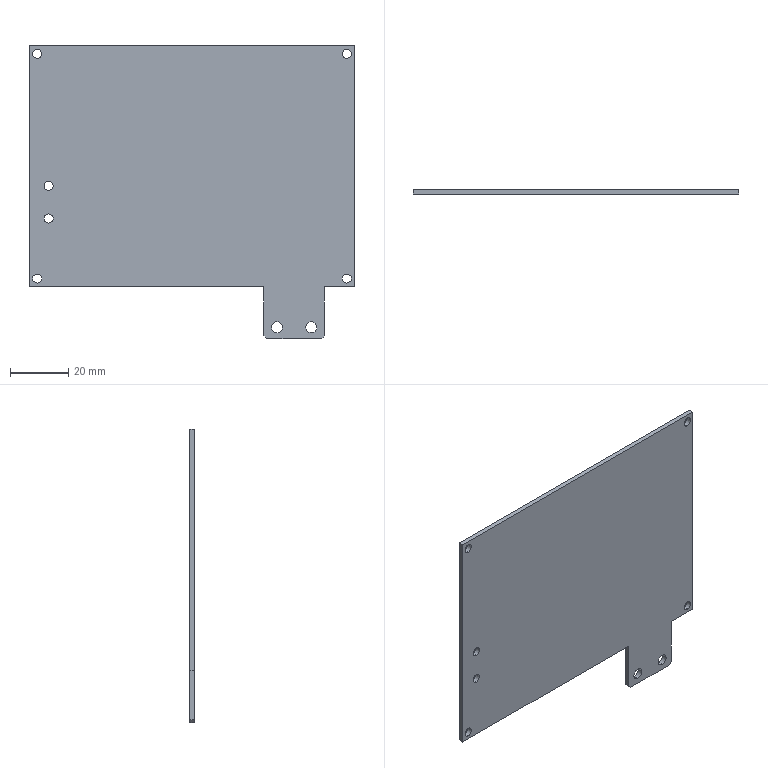Part | SolidWorks | features Extrusion 1 | 1 solid | 28 faces | box 111.5 x 1.7 x 100.35 mm | volume 16166 mm3 | cylinder 16 | plane 12 | commonest cylinder face diameters 3.1 x12 3.8 x4
STEP:
#1=CARTESIAN_POINT('',(-49.1,1.7,-8.3));
#2=VERTEX_POINT('',#1);
#3=CARTESIAN_POINT('',(-49.1,1.7,-5.2));
#4=VERTEX_POINT('',#3);
#5=CARTESIAN_POINT('',(-49.1,1.7,-6.75));
#6=DIRECTION('',(0.,1.,0.));
#7=DIRECTION('',(0.,0.,1.));
#8=AXIS2_PLACEMENT_3D('',#5,#6,#7);
#9=CIRCLE('',#8,1.55);
#10=EDGE_CURVE('',#2,#4,#9,.T.);
#11=ORIENTED_EDGE('',*,*,#10,.T.);
#12=CARTESIAN_POINT('',(-49.1,0.,-5.2));
#13=VERTEX_POINT('',#12);
#14=CARTESIAN_POINT('',(-49.1,1.7,-5.2));
#15=DIRECTION('',(0.,-1.,0.));
#16=VECTOR('',#15,1000.);
#17=LINE('',#14,#16);
#18=EDGE_CURVE('',#4,#13,#17,.T.);
#19=ORIENTED_EDGE('',*,*,#18,.T.);
#20=CARTESIAN_POINT('',(-49.1,0.,-8.3));
#21=VERTEX_POINT('',#20);
#22=CARTESIAN_POINT('',(-49.1,0.,-6.75));
#23=DIRECTION('',(0.,1.,0.));
#24=DIRECTION('',(0.,0.,1.));
#25=AXIS2_PLACEMENT_3D('',#22,#23,#24);
#26=CIRCLE('',#25,1.55);
#27=EDGE_CURVE('',#21,#13,#26,.T.);
#28=ORIENTED_EDGE('',*,*,#27,.F.);
#29=CARTESIAN_POINT('',(-49.1,1.7,-8.3));
#30=DIRECTION('',(0.,-1.,0.));
#31=VECTOR('',#30,1000.);
#32=LINE('',#29,#31);
#33=EDGE_CURVE('',#2,#21,#32,.T.);
#34=ORIENTED_EDGE('',*,*,#33,.F.);
#35=EDGE_LOOP('',(#11,#19,#28,#34));
#36=FACE_OUTER_BOUND('',#35,.T.);
#37=CARTESIAN_POINT('',(-49.1,1.7,-6.75));
#38=DIRECTION('',(0.,-1.,0.));
#39=DIRECTION('',(0.,0.,-1.));
#40=AXIS2_PLACEMENT_3D('',#37,#38,#39);
#41=CYLINDRICAL_SURFACE('',#40,1.55);
#42=ADVANCED_FACE('',(#36),#41,.F.);
#43=CARTESIAN_POINT('',(-49.1,1.7,-19.5));
#44=VERTEX_POINT('',#43);
#45=CARTESIAN_POINT('',(-49.1,1.7,-16.4));
#46=VERTEX_POINT('',#45);
#47=CARTESIAN_POINT('',(-49.1,1.7,-17.95));
#48=DIRECTION('',(0.,1.,0.));
#49=DIRECTION('',(0.,0.,1.));
#50=AXIS2_PLACEMENT_3D('',#47,#48,#49);
#51=CIRCLE('',#50,1.55);
#52=EDGE_CURVE('',#44,#46,#51,.T.);
#53=ORIENTED_EDGE('',*,*,#52,.T.);
#54=CARTESIAN_POINT('',(-49.1,0.,-16.4));
#55=VERTEX_POINT('',#54);
#56=CARTESIAN_POINT('',(-49.1,1.7,-16.4));
#57=DIRECTION('',(0.,-1.,0.));
#58=VECTOR('',#57,1000.);
#59=LINE('',#56,#58);
#60=EDGE_CURVE('',#46,#55,#59,.T.);
#61=ORIENTED_EDGE('',*,*,#60,.T.);
#62=CARTESIAN_POINT('',(-49.1,0.,-19.5));
#63=VERTEX_POINT('',#62);
#64=CARTESIAN_POINT('',(-49.1,0.,-17.95));
#65=DIRECTION('',(0.,1.,0.));
#66=DIRECTION('',(0.,0.,1.));
#67=AXIS2_PLACEMENT_3D('',#64,#65,#66);
#68=CIRCLE('',#67,1.55);
#69=EDGE_CURVE('',#63,#55,#68,.T.);
#70=ORIENTED_EDGE('',*,*,#69,.F.);
#71=CARTESIAN_POINT('',(-49.1,1.7,-19.5));
#72=DIRECTION('',(0.,-1.,0.));
#73=VECTOR('',#72,1000.);
#74=LINE('',#71,#73);
#75=EDGE_CURVE('',#44,#63,#74,.T.);
#76=ORIENTED_EDGE('',*,*,#75,.F.);
#77=EDGE_LOOP('',(#53,#61,#70,#76));
#78=FACE_OUTER_BOUND('',#77,.T.);
#79=CARTESIAN_POINT('',(-49.1,1.7,-17.95));
#80=DIRECTION('',(0.,-1.,0.));
#81=DIRECTION('',(0.,0.,-1.));
#82=AXIS2_PLACEMENT_3D('',#79,#80,#81);
#83=CYLINDRICAL_SURFACE('',#82,1.55);
#84=ADVANCED_FACE('',(#78),#83,.F.);
#85=CARTESIAN_POINT('',(40.875,1.7,-57.05));
#86=VERTEX_POINT('',#85);
#87=CARTESIAN_POINT('',(40.875,1.7,-53.25));
#88=VERTEX_POINT('',#87);
#89=CARTESIAN_POINT('',(40.875,1.7,-55.15));
#90=DIRECTION('',(0.,1.,0.));
#91=DIRECTION('',(0.,0.,-1.));
#92=AXIS2_PLACEMENT_3D('',#89,#90,#91);
#93=CIRCLE('',#92,1.9);
#94=EDGE_CURVE('',#86,#88,#93,.T.);
#95=ORIENTED_EDGE('',*,*,#94,.T.);
#96=CARTESIAN_POINT('',(40.875,0.,-53.25));
#97=VERTEX_POINT('',#96);
#98=CARTESIAN_POINT('',(40.875,1.7,-53.25));
#99=DIRECTION('',(0.,-1.,0.));
#100=VECTOR('',#99,1000.);
#101=LINE('',#98,#100);
#102=EDGE_CURVE('',#88,#97,#101,.T.);
#103=ORIENTED_EDGE('',*,*,#102,.T.);
#104=CARTESIAN_POINT('',(40.875,0.,-57.05));
#105=VERTEX_POINT('',#104);
#106=CARTESIAN_POINT('',(40.875,0.,-55.15));
#107=DIRECTION('',(0.,1.,0.));
#108=DIRECTION('',(0.,0.,-1.));
#109=AXIS2_PLACEMENT_3D('',#106,#107,#108);
#110=CIRCLE('',#109,1.9);
#111=EDGE_CURVE('',#105,#97,#110,.T.);
#112=ORIENTED_EDGE('',*,*,#111,.F.);
#113=CARTESIAN_POINT('',(40.875,1.7,-57.05));
#114=DIRECTION('',(0.,-1.,0.));
#115=VECTOR('',#114,1000.);
#116=LINE('',#113,#115);
#117=EDGE_CURVE('',#86,#105,#116,.T.);
#118=ORIENTED_EDGE('',*,*,#117,.F.);
#119=EDGE_LOOP('',(#95,#103,#112,#118));
#120=FACE_OUTER_BOUND('',#119,.T.);
#121=CARTESIAN_POINT('',(40.875,1.7,-55.15));
#122=DIRECTION('',(0.,-1.,0.));
#123=DIRECTION('',(0.,0.,-1.));
#124=AXIS2_PLACEMENT_3D('',#121,#122,#123);
#125=CYLINDRICAL_SURFACE('',#124,1.9);
#126=ADVANCED_FACE('',(#120),#125,.F.);
#127=CARTESIAN_POINT('',(29.075,1.7,-57.05));
#128=VERTEX_POINT('',#127);
#129=CARTESIAN_POINT('',(29.075,1.7,-53.25));
#130=VERTEX_POINT('',#129);
#131=CARTESIAN_POINT('',(29.075,1.7,-55.15));
#132=DIRECTION('',(0.,1.,0.));
#133=DIRECTION('',(0.,0.,1.));
#134=AXIS2_PLACEMENT_3D('',#131,#132,#133);
#135=CIRCLE('',#134,1.9);
#136=EDGE_CURVE('',#128,#130,#135,.T.);
#137=ORIENTED_EDGE('',*,*,#136,.T.);
#138=CARTESIAN_POINT('',(29.075,0.,-53.25));
#139=VERTEX_POINT('',#138);
#140=CARTESIAN_POINT('',(29.075,1.7,-53.25));
#141=DIRECTION('',(0.,-1.,0.));
#142=VECTOR('',#141,1000.);
#143=LINE('',#140,#142);
#144=EDGE_CURVE('',#130,#139,#143,.T.);
#145=ORIENTED_EDGE('',*,*,#144,.T.);
#146=CARTESIAN_POINT('',(29.075,0.,-57.05));
#147=VERTEX_POINT('',#146);
#148=CARTESIAN_POINT('',(29.075,0.,-55.15));
#149=DIRECTION('',(0.,1.,0.));
#150=DIRECTION('',(0.,0.,1.));
#151=AXIS2_PLACEMENT_3D('',#148,#149,#150);
#152=CIRCLE('',#151,1.9);
#153=EDGE_CURVE('',#147,#139,#152,.T.);
#154=ORIENTED_EDGE('',*,*,#153,.F.);
#155=CARTESIAN_POINT('',(29.075,1.7,-57.05));
#156=DIRECTION('',(0.,-1.,0.));
#157=VECTOR('',#156,1000.);
#158=LINE('',#155,#157);
#159=EDGE_CURVE('',#128,#147,#158,.T.);
#160=ORIENTED_EDGE('',*,*,#159,.F.);
#161=EDGE_LOOP('',(#137,#145,#154,#160));
#162=FACE_OUTER_BOUND('',#161,.T.);
#163=CARTESIAN_POINT('',(29.075,1.7,-55.15));
#164=DIRECTION('',(0.,-1.,0.));
#165=DIRECTION('',(0.,0.,-1.));
#166=AXIS2_PLACEMENT_3D('',#163,#164,#165);
#167=CYLINDRICAL_SURFACE('',#166,1.9);
#168=ADVANCED_FACE('',(#162),#167,.F.);
#169=CARTESIAN_POINT('',(-53.,1.7,36.95));
#170=VERTEX_POINT('',#169);
#171=CARTESIAN_POINT('',(-53.,1.7,40.05));
#172=VERTEX_POINT('',#171);
#173=CARTESIAN_POINT('',(-53.,1.7,38.5));
#174=DIRECTION('',(0.,1.,0.));
#175=DIRECTION('',(0.,0.,-1.));
#176=AXIS2_PLACEMENT_3D('',#173,#174,#175);
#177=CIRCLE('',#176,1.55);
#178=EDGE_CURVE('',#170,#172,#177,.T.);
#179=ORIENTED_EDGE('',*,*,#178,.T.);
#180=CARTESIAN_POINT('',(-53.,0.,40.05));
#181=VERTEX_POINT('',#180);
#182=CARTESIAN_POINT('',(-53.,1.7,40.05));
#183=DIRECTION('',(0.,-1.,0.));
#184=VECTOR('',#183,1000.);
#185=LINE('',#182,#184);
#186=EDGE_CURVE('',#172,#181,#185,.T.);
#187=ORIENTED_EDGE('',*,*,#186,.T.);
#188=CARTESIAN_POINT('',(-53.,0.,36.95));
#189=VERTEX_POINT('',#188);
#190=CARTESIAN_POINT('',(-53.,0.,38.5));
#191=DIRECTION('',(0.,1.,0.));
#192=DIRECTION('',(0.,0.,-1.));
#193=AXIS2_PLACEMENT_3D('',#190,#191,#192);
#194=CIRCLE('',#193,1.55);
#195=EDGE_CURVE('',#189,#181,#194,.T.);
#196=ORIENTED_EDGE('',*,*,#195,.F.);
#197=CARTESIAN_POINT('',(-53.,1.7,36.95));
#198=DIRECTION('',(0.,-1.,0.));
#199=VECTOR('',#198,1000.);
#200=LINE('',#197,#199);
#201=EDGE_CURVE('',#170,#189,#200,.T.);
#202=ORIENTED_EDGE('',*,*,#201,.F.);
#203=EDGE_LOOP('',(#179,#187,#196,#202));
#204=FACE_OUTER_BOUND('',#203,.T.);
#205=CARTESIAN_POINT('',(-53.,1.7,38.5));
#206=DIRECTION('',(0.,-1.,0.));
#207=DIRECTION('',(0.,0.,-1.));
#208=AXIS2_PLACEMENT_3D('',#205,#206,#207);
#209=CYLINDRICAL_SURFACE('',#208,1.55);
#210=ADVANCED_FACE('',(#204),#209,.F.);
#211=CARTESIAN_POINT('',(53.,1.7,36.95));
#212=VERTEX_POINT('',#211);
#213=CARTESIAN_POINT('',(53.,1.7,40.05));
#214=VERTEX_POINT('',#213);
#215=CARTESIAN_POINT('',(53.,1.7,38.5));
#216=DIRECTION('',(0.,1.,0.));
#217=DIRECTION('',(0.,0.,1.));
#218=AXIS2_PLACEMENT_3D('',#215,#216,#217);
#219=CIRCLE('',#218,1.55);
#220=EDGE_CURVE('',#212,#214,#219,.T.);
#221=ORIENTED_EDGE('',*,*,#220,.T.);
#222=CARTESIAN_POINT('',(53.,0.,40.05));
#223=VERTEX_POINT('',#222);
#224=CARTESIAN_POINT('',(53.,1.7,40.05));
#225=DIRECTION('',(0.,-1.,0.));
#226=VECTOR('',#225,1000.);
#227=LINE('',#224,#226);
#228=EDGE_CURVE('',#214,#223,#227,.T.);
#229=ORIENTED_EDGE('',*,*,#228,.T.);
#230=CARTESIAN_POINT('',(53.,0.,36.95));
#231=VERTEX_POINT('',#230);
#232=CARTESIAN_POINT('',(53.,0.,38.5));
#233=DIRECTION('',(0.,1.,0.));
#234=DIRECTION('',(0.,0.,1.));
#235=AXIS2_PLACEMENT_3D('',#232,#233,#234);
#236=CIRCLE('',#235,1.55);
#237=EDGE_CURVE('',#231,#223,#236,.T.);
#238=ORIENTED_EDGE('',*,*,#237,.F.);
#239=CARTESIAN_POINT('',(53.,1.7,36.95));
#240=DIRECTION('',(0.,-1.,0.));
#241=VECTOR('',#240,1000.);
#242=LINE('',#239,#241);
#243=EDGE_CURVE('',#212,#231,#242,.T.);
#244=ORIENTED_EDGE('',*,*,#243,.F.);
#245=EDGE_LOOP('',(#221,#229,#238,#244));
#246=FACE_OUTER_BOUND('',#245,.T.);
#247=CARTESIAN_POINT('',(53.,1.7,38.5));
#248=DIRECTION('',(0.,-1.,0.));
#249=DIRECTION('',(0.,0.,-1.));
#250=AXIS2_PLACEMENT_3D('',#247,#248,#249);
#251=CYLINDRICAL_SURFACE('',#250,1.55);
#252=ADVANCED_FACE('',(#246),#251,.F.);
#253=CARTESIAN_POINT('',(53.,1.7,-40.05));
#254=VERTEX_POINT('',#253);
#255=CARTESIAN_POINT('',(53.,1.7,-36.95));
#256=VERTEX_POINT('',#255);
#257=CARTESIAN_POINT('',(53.,1.7,-38.5));
#258=DIRECTION('',(0.,1.,0.));
#259=DIRECTION('',(0.,0.,-1.));
#260=AXIS2_PLACEMENT_3D('',#257,#258,#259);
#261=CIRCLE('',#260,1.55);
#262=EDGE_CURVE('',#254,#256,#261,.T.);
#263=ORIENTED_EDGE('',*,*,#262,.T.);
#264=CARTESIAN_POINT('',(53.,0.,-36.95));
#265=VERTEX_POINT('',#264);
#266=CARTESIAN_POINT('',(53.,1.7,-36.95));
#267=DIRECTION('',(0.,-1.,0.));
#268=VECTOR('',#267,1000.);
#269=LINE('',#266,#268);
#270=EDGE_CURVE('',#256,#265,#269,.T.);
#271=ORIENTED_EDGE('',*,*,#270,.T.);
#272=CARTESIAN_POINT('',(53.,0.,-40.05));
#273=VERTEX_POINT('',#272);
#274=CARTESIAN_POINT('',(53.,0.,-38.5));
#275=DIRECTION('',(0.,1.,0.));
#276=DIRECTION('',(0.,0.,-1.));
#277=AXIS2_PLACEMENT_3D('',#274,#275,#276);
#278=CIRCLE('',#277,1.55);
#279=EDGE_CURVE('',#273,#265,#278,.T.);
#280=ORIENTED_EDGE('',*,*,#279,.F.);
#281=CARTESIAN_POINT('',(53.,1.7,-40.05));
#282=DIRECTION('',(0.,-1.,0.));
#283=VECTOR('',#282,1000.);
#284=LINE('',#281,#283);
#285=EDGE_CURVE('',#254,#273,#284,.T.);
#286=ORIENTED_EDGE('',*,*,#285,.F.);
#287=EDGE_LOOP('',(#263,#271,#280,#286));
#288=FACE_OUTER_BOUND('',#287,.T.);
#289=CARTESIAN_POINT('',(53.,1.7,-38.5));
#290=DIRECTION('',(0.,-1.,0.));
#291=DIRECTION('',(0.,0.,-1.));
#292=AXIS2_PLACEMENT_3D('',#289,#290,#291);
#293=CYLINDRICAL_SURFACE('',#292,1.55);
#294=ADVANCED_FACE('',(#288),#293,.F.);
#295=CARTESIAN_POINT('',(-53.,1.7,-40.05));
#296=VERTEX_POINT('',#295);
#297=CARTESIAN_POINT('',(-53.,1.7,-36.95));
#298=VERTEX_POINT('',#297);
#299=CARTESIAN_POINT('',(-53.,1.7,-38.5));
#300=DIRECTION('',(0.,1.,0.));
#301=DIRECTION('',(0.,0.,1.));
#302=AXIS2_PLACEMENT_3D('',#299,#300,#301);
#303=CIRCLE('',#302,1.55);
#304=EDGE_CURVE('',#296,#298,#303,.T.);
#305=ORIENTED_EDGE('',*,*,#304,.T.);
#306=CARTESIAN_POINT('',(-53.,0.,-36.95));
#307=VERTEX_POINT('',#306);
#308=CARTESIAN_POINT('',(-53.,1.7,-36.95));
#309=DIRECTION('',(0.,-1.,0.));
#310=VECTOR('',#309,1000.);
#311=LINE('',#308,#310);
#312=EDGE_CURVE('',#298,#307,#311,.T.);
#313=ORIENTED_EDGE('',*,*,#312,.T.);
#314=CARTESIAN_POINT('',(-53.,0.,-40.05));
#315=VERTEX_POINT('',#314);
#316=CARTESIAN_POINT('',(-53.,0.,-38.5));
#317=DIRECTION('',(0.,1.,0.));
#318=DIRECTION('',(0.,0.,1.));
#319=AXIS2_PLACEMENT_3D('',#316,#317,#318);
#320=CIRCLE('',#319,1.55);
#321=EDGE_CURVE('',#315,#307,#320,.T.);
#322=ORIENTED_EDGE('',*,*,#321,.F.);
#323=CARTESIAN_POINT('',(-53.,1.7,-40.05));
#324=DIRECTION('',(0.,-1.,0.));
#325=VECTOR('',#324,1000.);
#326=LINE('',#323,#325);
#327=EDGE_CURVE('',#296,#315,#326,.T.);
#328=ORIENTED_EDGE('',*,*,#327,.F.);
#329=EDGE_LOOP('',(#305,#313,#322,#328));
#330=FACE_OUTER_BOUND('',#329,.T.);
#331=CARTESIAN_POINT('',(-53.,1.7,-38.5));
#332=DIRECTION('',(0.,-1.,0.));
#333=DIRECTION('',(0.,0.,-1.));
#334=AXIS2_PLACEMENT_3D('',#331,#332,#333);
#335=CYLINDRICAL_SURFACE('',#334,1.55);
#336=ADVANCED_FACE('',(#330),#335,.F.);
#337=ORIENTED_EDGE('',*,*,#52,.F.);
#338=CARTESIAN_POINT('',(-49.1,1.7,-17.95));
#339=DIRECTION('',(0.,1.,0.));
#340=DIRECTION('',(0.,0.,1.));
#341=AXIS2_PLACEMENT_3D('',#338,#339,#340);
#342=CIRCLE('',#341,1.55);
#343=EDGE_CURVE('',#46,#44,#342,.T.);
#344=ORIENTED_EDGE('',*,*,#343,.F.);
#345=EDGE_LOOP('',(#337,#344));
#346=FACE_BOUND('',#345,.T.);
#347=ORIENTED_EDGE('',*,*,#136,.F.);
#348=CARTESIAN_POINT('',(29.075,1.7,-55.15));
#349=DIRECTION('',(0.,1.,0.));
#350=DIRECTION('',(0.,0.,1.));
#351=AXIS2_PLACEMENT_3D('',#348,#349,#350);
#352=CIRCLE('',#351,1.9);
#353=EDGE_CURVE('',#130,#128,#352,.T.);
#354=ORIENTED_EDGE('',*,*,#353,.F.);
#355=EDGE_LOOP('',(#347,#354));
#356=FACE_BOUND('',#355,.T.);
#357=ORIENTED_EDGE('',*,*,#220,.F.);
#358=CARTESIAN_POINT('',(53.,1.7,38.5));
#359=DIRECTION('',(0.,1.,0.));
#360=DIRECTION('',(0.,0.,1.));
#361=AXIS2_PLACEMENT_3D('',#358,#359,#360);
#362=CIRCLE('',#361,1.55);
#363=EDGE_CURVE('',#214,#212,#362,.T.);
#364=ORIENTED_EDGE('',*,*,#363,.F.);
#365=EDGE_LOOP('',(#357,#364));
#366=FACE_BOUND('',#365,.T.);
#367=ORIENTED_EDGE('',*,*,#304,.F.);
#368=CARTESIAN_POINT('',(-53.,1.7,-38.5));
#369=DIRECTION('',(0.,1.,0.));
#370=DIRECTION('',(0.,0.,1.));
#371=AXIS2_PLACEMENT_3D('',#368,#369,#370);
#372=CIRCLE('',#371,1.55);
#373=EDGE_CURVE('',#298,#296,#372,.T.);
#374=ORIENTED_EDGE('',*,*,#373,.F.);
#375=EDGE_LOOP('',(#367,#374));
#376=FACE_BOUND('',#375,.T.);
#377=CARTESIAN_POINT('',(55.75,1.7,-41.3));
#378=VERTEX_POINT('',#377);
#379=CARTESIAN_POINT('',(45.35,1.7,-41.3));
#380=VERTEX_POINT('',#379);
#381=CARTESIAN_POINT('',(45.35,1.7,-41.3));
#382=DIRECTION('',(-1.,0.,0.));
#383=VECTOR('',#382,1000.);
#384=LINE('',#381,#383);
#385=EDGE_CURVE('',#378,#380,#384,.T.);
#386=ORIENTED_EDGE('',*,*,#385,.T.);
#387=CARTESIAN_POINT('',(45.35,1.7,-58.05));
#388=VERTEX_POINT('',#387);
#389=CARTESIAN_POINT('',(45.35,1.7,-58.05));
#390=DIRECTION('',(0.,0.,-1.));
#391=VECTOR('',#390,1000.);
#392=LINE('',#389,#391);
#393=EDGE_CURVE('',#380,#388,#392,.T.);
#394=ORIENTED_EDGE('',*,*,#393,.T.);
#395=CARTESIAN_POINT('',(44.35,1.7,-59.05));
#396=VERTEX_POINT('',#395);
#397=CARTESIAN_POINT('',(44.35,1.7,-59.05));
#398=DIRECTION('',(-0.7071,0.,-0.7071));
#399=VECTOR('',#398,1000.);
#400=LINE('',#397,#399);
#401=EDGE_CURVE('',#388,#396,#400,.T.);
#402=ORIENTED_EDGE('',*,*,#401,.T.);
#403=CARTESIAN_POINT('',(25.6,1.7,-59.05));
#404=VERTEX_POINT('',#403);
#405=CARTESIAN_POINT('',(25.6,1.7,-59.05));
#406=DIRECTION('',(-1.,0.,0.));
#407=VECTOR('',#406,1000.);
#408=LINE('',#405,#407);
#409=EDGE_CURVE('',#396,#404,#408,.T.);
#410=ORIENTED_EDGE('',*,*,#409,.T.);
#411=CARTESIAN_POINT('',(24.6,1.7,-58.05));
#412=VERTEX_POINT('',#411);
#413=CARTESIAN_POINT('',(24.6,1.7,-58.05));
#414=DIRECTION('',(-0.7071,0.,0.7071));
#415=VECTOR('',#414,1000.);
#416=LINE('',#413,#415);
#417=EDGE_CURVE('',#404,#412,#416,.T.);
#418=ORIENTED_EDGE('',*,*,#417,.T.);
#419=CARTESIAN_POINT('',(24.6,1.7,-41.3));
#420=VERTEX_POINT('',#419);
#421=CARTESIAN_POINT('',(24.6,1.7,-41.3));
#422=DIRECTION('',(0.,0.,1.));
#423=VECTOR('',#422,1000.);
#424=LINE('',#421,#423);
#425=EDGE_CURVE('',#412,#420,#424,.T.);
#426=ORIENTED_EDGE('',*,*,#425,.T.);
#427=CARTESIAN_POINT('',(-55.75,1.7,-41.3));
#428=VERTEX_POINT('',#427);
#429=CARTESIAN_POINT('',(-55.75,1.7,-41.3));
#430=DIRECTION('',(-1.,0.,0.));
#431=VECTOR('',#430,1000.);
#432=LINE('',#429,#431);
#433=EDGE_CURVE('',#420,#428,#432,.T.);
#434=ORIENTED_EDGE('',*,*,#433,.T.);
#435=CARTESIAN_POINT('',(-55.75,1.7,41.3));
#436=VERTEX_POINT('',#435);
#437=CARTESIAN_POINT('',(-55.75,1.7,41.3));
#438=DIRECTION('',(0.,0.,1.));
#439=VECTOR('',#438,1000.);
#440=LINE('',#437,#439);
#441=EDGE_CURVE('',#428,#436,#440,.T.);
#442=ORIENTED_EDGE('',*,*,#441,.T.);
#443=CARTESIAN_POINT('',(55.75,1.7,41.3));
#444=VERTEX_POINT('',#443);
#445=CARTESIAN_POINT('',(-55.75,1.7,41.3));
#446=DIRECTION('',(1.,0.,0.));
#447=VECTOR('',#446,1000.);
#448=LINE('',#445,#447);
#449=EDGE_CURVE('',#436,#444,#448,.T.);
#450=ORIENTED_EDGE('',*,*,#449,.T.);
#451=CARTESIAN_POINT('',(55.75,1.7,41.3));
#452=DIRECTION('',(0.,0.,-1.));
#453=VECTOR('',#452,1000.);
#454=LINE('',#451,#453);
#455=EDGE_CURVE('',#444,#378,#454,.T.);
#456=ORIENTED_EDGE('',*,*,#455,.T.);
#457=EDGE_LOOP('',(#386,#394,#402,#410,#418,#426,#434,#442,#450,#456));
#458=FACE_OUTER_BOUND('',#457,.T.);
#459=ORIENTED_EDGE('',*,*,#262,.F.);
#460=CARTESIAN_POINT('',(53.,1.7,-38.5));
#461=DIRECTION('',(0.,1.,0.));
#462=DIRECTION('',(0.,0.,-1.));
#463=AXIS2_PLACEMENT_3D('',#460,#461,#462);
#464=CIRCLE('',#463,1.55);
#465=EDGE_CURVE('',#256,#254,#464,.T.);
#466=ORIENTED_EDGE('',*,*,#465,.F.);
#467=EDGE_LOOP('',(#459,#466));
#468=FACE_BOUND('',#467,.T.);
#469=ORIENTED_EDGE('',*,*,#178,.F.);
#470=CARTESIAN_POINT('',(-53.,1.7,38.5));
#471=DIRECTION('',(0.,1.,0.));
#472=DIRECTION('',(0.,0.,-1.));
#473=AXIS2_PLACEMENT_3D('',#470,#471,#472);
#474=CIRCLE('',#473,1.55);
#475=EDGE_CURVE('',#172,#170,#474,.T.);
#476=ORIENTED_EDGE('',*,*,#475,.F.);
#477=EDGE_LOOP('',(#469,#476));
#478=FACE_BOUND('',#477,.T.);
#479=ORIENTED_EDGE('',*,*,#94,.F.);
#480=CARTESIAN_POINT('',(40.875,1.7,-55.15));
#481=DIRECTION('',(0.,1.,0.));
#482=DIRECTION('',(0.,0.,-1.));
#483=AXIS2_PLACEMENT_3D('',#480,#481,#482);
#484=CIRCLE('',#483,1.9);
#485=EDGE_CURVE('',#88,#86,#484,.T.);
#486=ORIENTED_EDGE('',*,*,#485,.F.);
#487=EDGE_LOOP('',(#479,#486));
#488=FACE_BOUND('',#487,.T.);
#489=ORIENTED_EDGE('',*,*,#10,.F.);
#490=CARTESIAN_POINT('',(-49.1,1.7,-6.75));
#491=DIRECTION('',(0.,1.,0.));
#492=DIRECTION('',(0.,0.,1.));
#493=AXIS2_PLACEMENT_3D('',#490,#491,#492);
#494=CIRCLE('',#493,1.55);
#495=EDGE_CURVE('',#4,#2,#494,.T.);
#496=ORIENTED_EDGE('',*,*,#495,.F.);
#497=EDGE_LOOP('',(#489,#496));
#498=FACE_BOUND('',#497,.T.);
#499=CARTESIAN_POINT('',(0.,1.7,0.));
#500=DIRECTION('',(0.,1.,0.));
#501=DIRECTION('',(0.,0.,1.));
#502=AXIS2_PLACEMENT_3D('',#499,#500,#501);
#503=PLANE('',#502);
#504=ADVANCED_FACE('',(#346,#356,#366,#376,#458,#468,#478,#488,#498),#503,.T.);
#505=ORIENTED_EDGE('',*,*,#69,.T.);
#506=CARTESIAN_POINT('',(-49.1,0.,-17.95));
#507=DIRECTION('',(0.,1.,0.));
#508=DIRECTION('',(0.,0.,1.));
#509=AXIS2_PLACEMENT_3D('',#506,#507,#508);
#510=CIRCLE('',#509,1.55);
#511=EDGE_CURVE('',#55,#63,#510,.T.);
#512=ORIENTED_EDGE('',*,*,#511,.T.);
#513=EDGE_LOOP('',(#505,#512));
#514=FACE_BOUND('',#513,.T.);
#515=ORIENTED_EDGE('',*,*,#153,.T.);
#516=CARTESIAN_POINT('',(29.075,0.,-55.15));
#517=DIRECTION('',(0.,1.,0.));
#518=DIRECTION('',(0.,0.,1.));
#519=AXIS2_PLACEMENT_3D('',#516,#517,#518);
#520=CIRCLE('',#519,1.9);
#521=EDGE_CURVE('',#139,#147,#520,.T.);
#522=ORIENTED_EDGE('',*,*,#521,.T.);
#523=EDGE_LOOP('',(#515,#522));
#524=FACE_BOUND('',#523,.T.);
#525=ORIENTED_EDGE('',*,*,#237,.T.);
#526=CARTESIAN_POINT('',(53.,0.,38.5));
#527=DIRECTION('',(0.,1.,0.));
#528=DIRECTION('',(0.,0.,1.));
#529=AXIS2_PLACEMENT_3D('',#526,#527,#528);
#530=CIRCLE('',#529,1.55);
#531=EDGE_CURVE('',#223,#231,#530,.T.);
#532=ORIENTED_EDGE('',*,*,#531,.T.);
#533=EDGE_LOOP('',(#525,#532));
#534=FACE_BOUND('',#533,.T.);
#535=ORIENTED_EDGE('',*,*,#321,.T.);
#536=CARTESIAN_POINT('',(-53.,0.,-38.5));
#537=DIRECTION('',(0.,1.,0.));
#538=DIRECTION('',(0.,0.,1.));
#539=AXIS2_PLACEMENT_3D('',#536,#537,#538);
#540=CIRCLE('',#539,1.55);
#541=EDGE_CURVE('',#307,#315,#540,.T.);
#542=ORIENTED_EDGE('',*,*,#541,.T.);
#543=EDGE_LOOP('',(#535,#542));
#544=FACE_BOUND('',#543,.T.);
#545=CARTESIAN_POINT('',(55.75,0.,-41.3));
#546=VERTEX_POINT('',#545);
#547=CARTESIAN_POINT('',(45.35,0.,-41.3));
#548=VERTEX_POINT('',#547);
#549=CARTESIAN_POINT('',(45.35,0.,-41.3));
#550=DIRECTION('',(-1.,0.,0.));
#551=VECTOR('',#550,1000.);
#552=LINE('',#549,#551);
#553=EDGE_CURVE('',#546,#548,#552,.T.);
#554=ORIENTED_EDGE('',*,*,#553,.F.);
#555=CARTESIAN_POINT('',(55.75,0.,41.3));
#556=VERTEX_POINT('',#555);
#557=CARTESIAN_POINT('',(55.75,0.,41.3));
#558=DIRECTION('',(0.,0.,-1.));
#559=VECTOR('',#558,1000.);
#560=LINE('',#557,#559);
#561=EDGE_CURVE('',#556,#546,#560,.T.);
#562=ORIENTED_EDGE('',*,*,#561,.F.);
#563=CARTESIAN_POINT('',(-55.75,0.,41.3));
#564=VERTEX_POINT('',#563);
#565=CARTESIAN_POINT('',(-55.75,0.,41.3));
#566=DIRECTION('',(1.,0.,0.));
#567=VECTOR('',#566,1000.);
#568=LINE('',#565,#567);
#569=EDGE_CURVE('',#564,#556,#568,.T.);
#570=ORIENTED_EDGE('',*,*,#569,.F.);
#571=CARTESIAN_POINT('',(-55.75,0.,-41.3));
#572=VERTEX_POINT('',#571);
#573=CARTESIAN_POINT('',(-55.75,0.,41.3));
#574=DIRECTION('',(0.,0.,1.));
#575=VECTOR('',#574,1000.);
#576=LINE('',#573,#575);
#577=EDGE_CURVE('',#572,#564,#576,.T.);
#578=ORIENTED_EDGE('',*,*,#577,.F.);
#579=CARTESIAN_POINT('',(24.6,0.,-41.3));
#580=VERTEX_POINT('',#579);
#581=CARTESIAN_POINT('',(-55.75,0.,-41.3));
#582=DIRECTION('',(-1.,0.,0.));
#583=VECTOR('',#582,1000.);
#584=LINE('',#581,#583);
#585=EDGE_CURVE('',#580,#572,#584,.T.);
#586=ORIENTED_EDGE('',*,*,#585,.F.);
#587=CARTESIAN_POINT('',(24.6,0.,-58.05));
#588=VERTEX_POINT('',#587);
#589=CARTESIAN_POINT('',(24.6,0.,-41.3));
#590=DIRECTION('',(0.,0.,1.));
#591=VECTOR('',#590,1000.);
#592=LINE('',#589,#591);
#593=EDGE_CURVE('',#588,#580,#592,.T.);
#594=ORIENTED_EDGE('',*,*,#593,.F.);
#595=CARTESIAN_POINT('',(25.6,0.,-59.05));
#596=VERTEX_POINT('',#595);
#597=CARTESIAN_POINT('',(24.6,0.,-58.05));
#598=DIRECTION('',(-0.7071,0.,0.7071));
#599=VECTOR('',#598,1000.);
#600=LINE('',#597,#599);
#601=EDGE_CURVE('',#596,#588,#600,.T.);
#602=ORIENTED_EDGE('',*,*,#601,.F.);
#603=CARTESIAN_POINT('',(44.35,0.,-59.05));
#604=VERTEX_POINT('',#603);
#605=CARTESIAN_POINT('',(25.6,0.,-59.05));
#606=DIRECTION('',(-1.,0.,0.));
#607=VECTOR('',#606,1000.);
#608=LINE('',#605,#607);
#609=EDGE_CURVE('',#604,#596,#608,.T.);
#610=ORIENTED_EDGE('',*,*,#609,.F.);
#611=CARTESIAN_POINT('',(45.35,0.,-58.05));
#612=VERTEX_POINT('',#611);
#613=CARTESIAN_POINT('',(44.35,0.,-59.05));
#614=DIRECTION('',(-0.7071,0.,-0.7071));
#615=VECTOR('',#614,1000.);
#616=LINE('',#613,#615);
#617=EDGE_CURVE('',#612,#604,#616,.T.);
#618=ORIENTED_EDGE('',*,*,#617,.F.);
#619=CARTESIAN_POINT('',(45.35,0.,-58.05));
#620=DIRECTION('',(0.,0.,-1.));
#621=VECTOR('',#620,1000.);
#622=LINE('',#619,#621);
#623=EDGE_CURVE('',#548,#612,#622,.T.);
#624=ORIENTED_EDGE('',*,*,#623,.F.);
#625=EDGE_LOOP('',(#554,#562,#570,#578,#586,#594,#602,#610,#618,#624));
#626=FACE_OUTER_BOUND('',#625,.T.);
#627=ORIENTED_EDGE('',*,*,#279,.T.);
#628=CARTESIAN_POINT('',(53.,0.,-38.5));
#629=DIRECTION('',(0.,1.,0.));
#630=DIRECTION('',(0.,0.,-1.));
#631=AXIS2_PLACEMENT_3D('',#628,#629,#630);
#632=CIRCLE('',#631,1.55);
#633=EDGE_CURVE('',#265,#273,#632,.T.);
#634=ORIENTED_EDGE('',*,*,#633,.T.);
#635=EDGE_LOOP('',(#627,#634));
#636=FACE_BOUND('',#635,.T.);
#637=ORIENTED_EDGE('',*,*,#195,.T.);
#638=CARTESIAN_POINT('',(-53.,0.,38.5));
#639=DIRECTION('',(0.,1.,0.));
#640=DIRECTION('',(0.,0.,-1.));
#641=AXIS2_PLACEMENT_3D('',#638,#639,#640);
#642=CIRCLE('',#641,1.55);
#643=EDGE_CURVE('',#181,#189,#642,.T.);
#644=ORIENTED_EDGE('',*,*,#643,.T.);
#645=EDGE_LOOP('',(#637,#644));
#646=FACE_BOUND('',#645,.T.);
#647=ORIENTED_EDGE('',*,*,#111,.T.);
#648=CARTESIAN_POINT('',(40.875,0.,-55.15));
#649=DIRECTION('',(0.,1.,0.));
#650=DIRECTION('',(0.,0.,-1.));
#651=AXIS2_PLACEMENT_3D('',#648,#649,#650);
#652=CIRCLE('',#651,1.9);
#653=EDGE_CURVE('',#97,#105,#652,.T.);
#654=ORIENTED_EDGE('',*,*,#653,.T.);
#655=EDGE_LOOP('',(#647,#654));
#656=FACE_BOUND('',#655,.T.);
#657=ORIENTED_EDGE('',*,*,#27,.T.);
#658=CARTESIAN_POINT('',(-49.1,0.,-6.75));
#659=DIRECTION('',(0.,1.,0.));
#660=DIRECTION('',(0.,0.,1.));
#661=AXIS2_PLACEMENT_3D('',#658,#659,#660);
#662=CIRCLE('',#661,1.55);
#663=EDGE_CURVE('',#13,#21,#662,.T.);
#664=ORIENTED_EDGE('',*,*,#663,.T.);
#665=EDGE_LOOP('',(#657,#664));
#666=FACE_BOUND('',#665,.T.);
#667=CARTESIAN_POINT('',(0.,0.,0.));
#668=DIRECTION('',(0.,1.,0.));
#669=DIRECTION('',(0.,0.,1.));
#670=AXIS2_PLACEMENT_3D('',#667,#668,#669);
#671=PLANE('',#670);
#672=ADVANCED_FACE('',(#514,#524,#534,#544,#626,#636,#646,#656,#666),#671,.F.);
#673=ORIENTED_EDGE('',*,*,#553,.T.);
#674=CARTESIAN_POINT('',(45.35,1.7,-41.3));
#675=DIRECTION('',(0.,-1.,0.));
#676=VECTOR('',#675,1000.);
#677=LINE('',#674,#676);
#678=EDGE_CURVE('',#380,#548,#677,.T.);
#679=ORIENTED_EDGE('',*,*,#678,.F.);
#680=ORIENTED_EDGE('',*,*,#385,.F.);
#681=CARTESIAN_POINT('',(55.75,1.7,-41.3));
#682=DIRECTION('',(0.,-1.,0.));
#683=VECTOR('',#682,1000.);
#684=LINE('',#681,#683);
#685=EDGE_CURVE('',#378,#546,#684,.T.);
#686=ORIENTED_EDGE('',*,*,#685,.T.);
#687=EDGE_LOOP('',(#673,#679,#680,#686));
#688=FACE_OUTER_BOUND('',#687,.T.);
#689=CARTESIAN_POINT('',(45.35,1.7,-41.3));
#690=DIRECTION('',(0.,0.,1.));
#691=DIRECTION('',(1.,0.,0.));
#692=AXIS2_PLACEMENT_3D('',#689,#690,#691);
#693=PLANE('',#692);
#694=ADVANCED_FACE('',(#688),#693,.F.);
#695=ORIENTED_EDGE('',*,*,#623,.T.);
#696=CARTESIAN_POINT('',(45.35,1.7,-58.05));
#697=DIRECTION('',(0.,-1.,0.));
#698=VECTOR('',#697,1000.);
#699=LINE('',#696,#698);
#700=EDGE_CURVE('',#388,#612,#699,.T.);
#701=ORIENTED_EDGE('',*,*,#700,.F.);
#702=ORIENTED_EDGE('',*,*,#393,.F.);
#703=ORIENTED_EDGE('',*,*,#678,.T.);
#704=EDGE_LOOP('',(#695,#701,#702,#703));
#705=FACE_OUTER_BOUND('',#704,.T.);
#706=CARTESIAN_POINT('',(45.35,1.7,-58.05));
#707=DIRECTION('',(-1.,0.,0.));
#708=DIRECTION('',(0.,0.,1.));
#709=AXIS2_PLACEMENT_3D('',#706,#707,#708);
#710=PLANE('',#709);
#711=ADVANCED_FACE('',(#705),#710,.F.);
#712=ORIENTED_EDGE('',*,*,#617,.T.);
#713=CARTESIAN_POINT('',(44.35,1.7,-59.05));
#714=DIRECTION('',(0.,-1.,0.));
#715=VECTOR('',#714,1000.);
#716=LINE('',#713,#715);
#717=EDGE_CURVE('',#396,#604,#716,.T.);
#718=ORIENTED_EDGE('',*,*,#717,.F.);
#719=ORIENTED_EDGE('',*,*,#401,.F.);
#720=ORIENTED_EDGE('',*,*,#700,.T.);
#721=EDGE_LOOP('',(#712,#718,#719,#720));
#722=FACE_OUTER_BOUND('',#721,.T.);
#723=CARTESIAN_POINT('',(44.35,1.7,-59.05));
#724=DIRECTION('',(-0.7071,0.,0.7071));
#725=DIRECTION('',(0.7071,0.,0.7071));
#726=AXIS2_PLACEMENT_3D('',#723,#724,#725);
#727=PLANE('',#726);
#728=ADVANCED_FACE('',(#722),#727,.F.);
#729=ORIENTED_EDGE('',*,*,#609,.T.);
#730=CARTESIAN_POINT('',(25.6,1.7,-59.05));
#731=DIRECTION('',(0.,-1.,0.));
#732=VECTOR('',#731,1000.);
#733=LINE('',#730,#732);
#734=EDGE_CURVE('',#404,#596,#733,.T.);
#735=ORIENTED_EDGE('',*,*,#734,.F.);
#736=ORIENTED_EDGE('',*,*,#409,.F.);
#737=ORIENTED_EDGE('',*,*,#717,.T.);
#738=EDGE_LOOP('',(#729,#735,#736,#737));
#739=FACE_OUTER_BOUND('',#738,.T.);
#740=CARTESIAN_POINT('',(25.6,1.7,-59.05));
#741=DIRECTION('',(0.,0.,1.));
#742=DIRECTION('',(1.,0.,0.));
#743=AXIS2_PLACEMENT_3D('',#740,#741,#742);
#744=PLANE('',#743);
#745=ADVANCED_FACE('',(#739),#744,.F.);
#746=ORIENTED_EDGE('',*,*,#601,.T.);
#747=CARTESIAN_POINT('',(24.6,1.7,-58.05));
#748=DIRECTION('',(0.,-1.,0.));
#749=VECTOR('',#748,1000.);
#750=LINE('',#747,#749);
#751=EDGE_CURVE('',#412,#588,#750,.T.);
#752=ORIENTED_EDGE('',*,*,#751,.F.);
#753=ORIENTED_EDGE('',*,*,#417,.F.);
#754=ORIENTED_EDGE('',*,*,#734,.T.);
#755=EDGE_LOOP('',(#746,#752,#753,#754));
#756=FACE_OUTER_BOUND('',#755,.T.);
#757=CARTESIAN_POINT('',(24.6,1.7,-58.05));
#758=DIRECTION('',(0.7071,0.,0.7071));
#759=DIRECTION('',(0.7071,0.,-0.7071));
#760=AXIS2_PLACEMENT_3D('',#757,#758,#759);
#761=PLANE('',#760);
#762=ADVANCED_FACE('',(#756),#761,.F.);
#763=ORIENTED_EDGE('',*,*,#593,.T.);
#764=CARTESIAN_POINT('',(24.6,1.7,-41.3));
#765=DIRECTION('',(0.,-1.,0.));
#766=VECTOR('',#765,1000.);
#767=LINE('',#764,#766);
#768=EDGE_CURVE('',#420,#580,#767,.T.);
#769=ORIENTED_EDGE('',*,*,#768,.F.);
#770=ORIENTED_EDGE('',*,*,#425,.F.);
#771=ORIENTED_EDGE('',*,*,#751,.T.);
#772=EDGE_LOOP('',(#763,#769,#770,#771));
#773=FACE_OUTER_BOUND('',#772,.T.);
#774=CARTESIAN_POINT('',(24.6,1.7,-41.3));
#775=DIRECTION('',(1.,0.,0.));
#776=DIRECTION('',(0.,0.,-1.));
#777=AXIS2_PLACEMENT_3D('',#774,#775,#776);
#778=PLANE('',#777);
#779=ADVANCED_FACE('',(#773),#778,.F.);
#780=ORIENTED_EDGE('',*,*,#585,.T.);
#781=CARTESIAN_POINT('',(-55.75,1.7,-41.3));
#782=DIRECTION('',(0.,-1.,0.));
#783=VECTOR('',#782,1000.);
#784=LINE('',#781,#783);
#785=EDGE_CURVE('',#428,#572,#784,.T.);
#786=ORIENTED_EDGE('',*,*,#785,.F.);
#787=ORIENTED_EDGE('',*,*,#433,.F.);
#788=ORIENTED_EDGE('',*,*,#768,.T.);
#789=EDGE_LOOP('',(#780,#786,#787,#788));
#790=FACE_OUTER_BOUND('',#789,.T.);
#791=CARTESIAN_POINT('',(-55.75,1.7,-41.3));
#792=DIRECTION('',(0.,0.,1.));
#793=DIRECTION('',(1.,0.,0.));
#794=AXIS2_PLACEMENT_3D('',#791,#792,#793);
#795=PLANE('',#794);
#796=ADVANCED_FACE('',(#790),#795,.F.);
#797=ORIENTED_EDGE('',*,*,#577,.T.);
#798=CARTESIAN_POINT('',(-55.75,1.7,41.3));
#799=DIRECTION('',(0.,-1.,0.));
#800=VECTOR('',#799,1000.);
#801=LINE('',#798,#800);
#802=EDGE_CURVE('',#436,#564,#801,.T.);
#803=ORIENTED_EDGE('',*,*,#802,.F.);
#804=ORIENTED_EDGE('',*,*,#441,.F.);
#805=ORIENTED_EDGE('',*,*,#785,.T.);
#806=EDGE_LOOP('',(#797,#803,#804,#805));
#807=FACE_OUTER_BOUND('',#806,.T.);
#808=CARTESIAN_POINT('',(-55.75,1.7,41.3));
#809=DIRECTION('',(1.,0.,0.));
#810=DIRECTION('',(0.,0.,-1.));
#811=AXIS2_PLACEMENT_3D('',#808,#809,#810);
#812=PLANE('',#811);
#813=ADVANCED_FACE('',(#807),#812,.F.);
#814=ORIENTED_EDGE('',*,*,#569,.T.);
#815=CARTESIAN_POINT('',(55.75,1.7,41.3));
#816=DIRECTION('',(0.,-1.,0.));
#817=VECTOR('',#816,1000.);
#818=LINE('',#815,#817);
#819=EDGE_CURVE('',#444,#556,#818,.T.);
#820=ORIENTED_EDGE('',*,*,#819,.F.);
#821=ORIENTED_EDGE('',*,*,#449,.F.);
#822=ORIENTED_EDGE('',*,*,#802,.T.);
#823=EDGE_LOOP('',(#814,#820,#821,#822));
#824=FACE_OUTER_BOUND('',#823,.T.);
#825=CARTESIAN_POINT('',(-55.75,1.7,41.3));
#826=DIRECTION('',(0.,0.,-1.));
#827=DIRECTION('',(-1.,0.,0.));
#828=AXIS2_PLACEMENT_3D('',#825,#826,#827);
#829=PLANE('',#828);
#830=ADVANCED_FACE('',(#824),#829,.F.);
#831=ORIENTED_EDGE('',*,*,#561,.T.);
#832=ORIENTED_EDGE('',*,*,#685,.F.);
#833=ORIENTED_EDGE('',*,*,#455,.F.);
#834=ORIENTED_EDGE('',*,*,#819,.T.);
#835=EDGE_LOOP('',(#831,#832,#833,#834));
#836=FACE_OUTER_BOUND('',#835,.T.);
#837=CARTESIAN_POINT('',(55.75,1.7,41.3));
#838=DIRECTION('',(-1.,0.,0.));
#839=DIRECTION('',(0.,0.,1.));
#840=AXIS2_PLACEMENT_3D('',#837,#838,#839);
#841=PLANE('',#840);
#842=ADVANCED_FACE('',(#836),#841,.F.);
#843=ORIENTED_EDGE('',*,*,#312,.F.);
#844=ORIENTED_EDGE('',*,*,#373,.T.);
#845=ORIENTED_EDGE('',*,*,#327,.T.);
#846=ORIENTED_EDGE('',*,*,#541,.F.);
#847=EDGE_LOOP('',(#843,#844,#845,#846));
#848=FACE_OUTER_BOUND('',#847,.T.);
#849=CARTESIAN_POINT('',(-53.,1.7,-38.5));
#850=DIRECTION('',(0.,-1.,0.));
#851=DIRECTION('',(0.,0.,-1.));
#852=AXIS2_PLACEMENT_3D('',#849,#850,#851);
#853=CYLINDRICAL_SURFACE('',#852,1.55);
#854=ADVANCED_FACE('',(#848),#853,.F.);
#855=ORIENTED_EDGE('',*,*,#270,.F.);
#856=ORIENTED_EDGE('',*,*,#465,.T.);
#857=ORIENTED_EDGE('',*,*,#285,.T.);
#858=ORIENTED_EDGE('',*,*,#633,.F.);
#859=EDGE_LOOP('',(#855,#856,#857,#858));
#860=FACE_OUTER_BOUND('',#859,.T.);
#861=CARTESIAN_POINT('',(53.,1.7,-38.5));
#862=DIRECTION('',(0.,-1.,0.));
#863=DIRECTION('',(0.,0.,-1.));
#864=AXIS2_PLACEMENT_3D('',#861,#862,#863);
#865=CYLINDRICAL_SURFACE('',#864,1.55);
#866=ADVANCED_FACE('',(#860),#865,.F.);
#867=ORIENTED_EDGE('',*,*,#228,.F.);
#868=ORIENTED_EDGE('',*,*,#363,.T.);
#869=ORIENTED_EDGE('',*,*,#243,.T.);
#870=ORIENTED_EDGE('',*,*,#531,.F.);
#871=EDGE_LOOP('',(#867,#868,#869,#870));
#872=FACE_OUTER_BOUND('',#871,.T.);
#873=CARTESIAN_POINT('',(53.,1.7,38.5));
#874=DIRECTION('',(0.,-1.,0.));
#875=DIRECTION('',(0.,0.,-1.));
#876=AXIS2_PLACEMENT_3D('',#873,#874,#875);
#877=CYLINDRICAL_SURFACE('',#876,1.55);
#878=ADVANCED_FACE('',(#872),#877,.F.);
#879=ORIENTED_EDGE('',*,*,#186,.F.);
#880=ORIENTED_EDGE('',*,*,#475,.T.);
#881=ORIENTED_EDGE('',*,*,#201,.T.);
#882=ORIENTED_EDGE('',*,*,#643,.F.);
#883=EDGE_LOOP('',(#879,#880,#881,#882));
#884=FACE_OUTER_BOUND('',#883,.T.);
#885=CARTESIAN_POINT('',(-53.,1.7,38.5));
#886=DIRECTION('',(0.,-1.,0.));
#887=DIRECTION('',(0.,0.,-1.));
#888=AXIS2_PLACEMENT_3D('',#885,#886,#887);
#889=CYLINDRICAL_SURFACE('',#888,1.55);
#890=ADVANCED_FACE('',(#884),#889,.F.);
#891=ORIENTED_EDGE('',*,*,#144,.F.);
#892=ORIENTED_EDGE('',*,*,#353,.T.);
#893=ORIENTED_EDGE('',*,*,#159,.T.);
#894=ORIENTED_EDGE('',*,*,#521,.F.);
#895=EDGE_LOOP('',(#891,#892,#893,#894));
#896=FACE_OUTER_BOUND('',#895,.T.);
#897=CARTESIAN_POINT('',(29.075,1.7,-55.15));
#898=DIRECTION('',(0.,-1.,0.));
#899=DIRECTION('',(0.,0.,-1.));
#900=AXIS2_PLACEMENT_3D('',#897,#898,#899);
#901=CYLINDRICAL_SURFACE('',#900,1.9);
#902=ADVANCED_FACE('',(#896),#901,.F.);
#903=ORIENTED_EDGE('',*,*,#102,.F.);
#904=ORIENTED_EDGE('',*,*,#485,.T.);
#905=ORIENTED_EDGE('',*,*,#117,.T.);
#906=ORIENTED_EDGE('',*,*,#653,.F.);
#907=EDGE_LOOP('',(#903,#904,#905,#906));
#908=FACE_OUTER_BOUND('',#907,.T.);
#909=CARTESIAN_POINT('',(40.875,1.7,-55.15));
#910=DIRECTION('',(0.,-1.,0.));
#911=DIRECTION('',(0.,0.,-1.));
#912=AXIS2_PLACEMENT_3D('',#909,#910,#911);
#913=CYLINDRICAL_SURFACE('',#912,1.9);
#914=ADVANCED_FACE('',(#908),#913,.F.);
#915=ORIENTED_EDGE('',*,*,#60,.F.);
#916=ORIENTED_EDGE('',*,*,#343,.T.);
#917=ORIENTED_EDGE('',*,*,#75,.T.);
#918=ORIENTED_EDGE('',*,*,#511,.F.);
#919=EDGE_LOOP('',(#915,#916,#917,#918));
#920=FACE_OUTER_BOUND('',#919,.T.);
#921=CARTESIAN_POINT('',(-49.1,1.7,-17.95));
#922=DIRECTION('',(0.,-1.,0.));
#923=DIRECTION('',(0.,0.,-1.));
#924=AXIS2_PLACEMENT_3D('',#921,#922,#923);
#925=CYLINDRICAL_SURFACE('',#924,1.55);
#926=ADVANCED_FACE('',(#920),#925,.F.);
#927=ORIENTED_EDGE('',*,*,#18,.F.);
#928=ORIENTED_EDGE('',*,*,#495,.T.);
#929=ORIENTED_EDGE('',*,*,#33,.T.);
#930=ORIENTED_EDGE('',*,*,#663,.F.);
#931=EDGE_LOOP('',(#927,#928,#929,#930));
#932=FACE_OUTER_BOUND('',#931,.T.);
#933=CARTESIAN_POINT('',(-49.1,1.7,-6.75));
#934=DIRECTION('',(0.,-1.,0.));
#935=DIRECTION('',(0.,0.,-1.));
#936=AXIS2_PLACEMENT_3D('',#933,#934,#935);
#937=CYLINDRICAL_SURFACE('',#936,1.55);
#938=ADVANCED_FACE('',(#932),#937,.F.);
#939=CLOSED_SHELL('',(#42,#84,#126,#168,#210,#252,#294,#336,#504,#672,#694,#711,#728,#745,#762,#779,#796,#813,#830,#842,#854,#866,#878,#890,#902,#914,#926,#938));
#940=MANIFOLD_SOLID_BREP('',#939);
#941=CARTESIAN_POINT('',(0.,0.,0.));
#942=DIRECTION('',(0.,0.,1.));
#943=DIRECTION('',(1.,0.,0.));
#944=AXIS2_PLACEMENT_3D('',#941,#942,#943);
#945=(LENGTH_UNIT()NAMED_UNIT(*)SI_UNIT(.MILLI.,.METRE.));
#946=UNCERTAINTY_MEASURE_WITH_UNIT(LENGTH_MEASURE(0.00001),#945,'','');
#947=(NAMED_UNIT(*)PLANE_ANGLE_UNIT()SI_UNIT($,.RADIAN.));
#948=(NAMED_UNIT(*)SI_UNIT($,.STERADIAN.)SOLID_ANGLE_UNIT());
#949=(GEOMETRIC_REPRESENTATION_CONTEXT(3)GLOBAL_UNCERTAINTY_ASSIGNED_CONTEXT((#946))GLOBAL_UNIT_ASSIGNED_CONTEXT((#945,#947,#948))REPRESENTATION_CONTEXT('',''));
#950=ADVANCED_BREP_SHAPE_REPRESENTATION('',(#940,#944),#949);